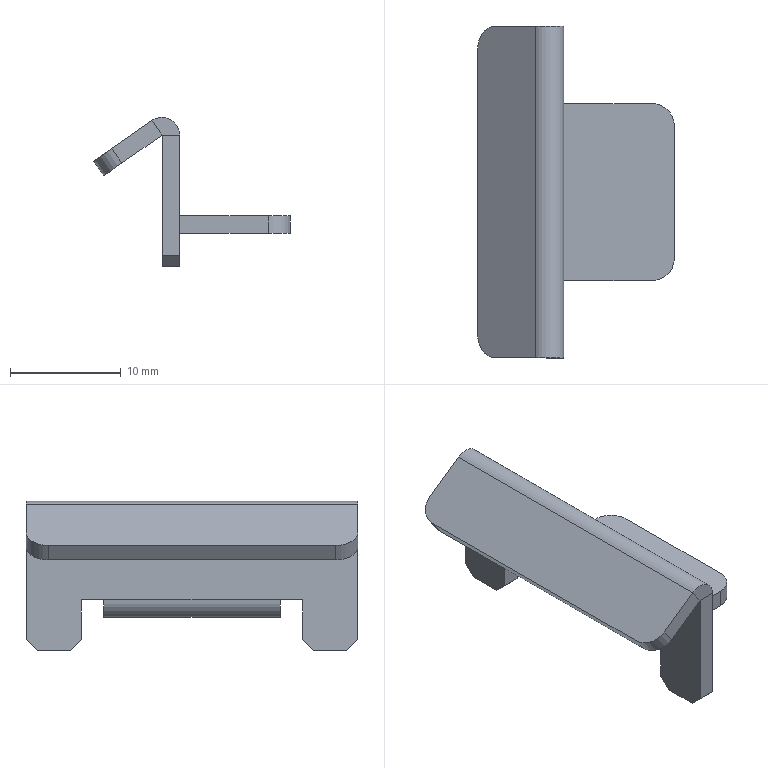Part | NX | features solid 2 | 1 solid | 34 faces | box 17.782 x 30 x 13.496 mm | volume 1096 mm3 | plane 28 | cylinder 6 | commonest cylinder face diameters 4 x4 3.2 x2
STEP:
#1=CARTESIAN_POINT('',(-290.6,942.6,-820.104));
#2=VERTEX_POINT('',#1);
#3=CARTESIAN_POINT('',(-290.6,942.6,-831.));
#4=VERTEX_POINT('',#3);
#5=CARTESIAN_POINT('',(-290.6,942.6,-820.104));
#6=DIRECTION('',(0.,0.,-1.));
#7=VECTOR('',#6,1000.);
#8=LINE('',#5,#7);
#9=EDGE_CURVE('',#2,#4,#8,.T.);
#10=ORIENTED_EDGE('',*,*,#9,.T.);
#11=CARTESIAN_POINT('',(-290.6,943.6,-832.));
#12=VERTEX_POINT('',#11);
#13=CARTESIAN_POINT('',(-290.6,943.6,-832.));
#14=DIRECTION('',(0.,-0.7071,0.7071));
#15=VECTOR('',#14,1000.);
#16=LINE('',#13,#15);
#17=EDGE_CURVE('',#12,#4,#16,.T.);
#18=ORIENTED_EDGE('',*,*,#17,.F.);
#19=CARTESIAN_POINT('',(-290.6,946.6,-832.));
#20=VERTEX_POINT('',#19);
#21=CARTESIAN_POINT('',(-290.6,943.6,-832.));
#22=DIRECTION('',(0.,1.,0.));
#23=VECTOR('',#22,1000.);
#24=LINE('',#21,#23);
#25=EDGE_CURVE('',#12,#20,#24,.T.);
#26=ORIENTED_EDGE('',*,*,#25,.T.);
#27=CARTESIAN_POINT('',(-290.6,947.6,-831.));
#28=VERTEX_POINT('',#27);
#29=CARTESIAN_POINT('',(-290.6,947.6,-831.));
#30=DIRECTION('',(0.,-0.7071,-0.7071));
#31=VECTOR('',#30,1000.);
#32=LINE('',#29,#31);
#33=EDGE_CURVE('',#28,#20,#32,.T.);
#34=ORIENTED_EDGE('',*,*,#33,.F.);
#35=CARTESIAN_POINT('',(-290.6,947.6,-827.4));
#36=VERTEX_POINT('',#35);
#37=CARTESIAN_POINT('',(-290.6,947.6,-831.));
#38=DIRECTION('',(0.,0.,1.));
#39=VECTOR('',#38,1000.);
#40=LINE('',#37,#39);
#41=EDGE_CURVE('',#28,#36,#40,.T.);
#42=ORIENTED_EDGE('',*,*,#41,.T.);
#43=CARTESIAN_POINT('',(-290.6,949.6,-827.4));
#44=VERTEX_POINT('',#43);
#45=CARTESIAN_POINT('',(-290.6,947.6,-827.4));
#46=DIRECTION('',(0.,1.,0.));
#47=VECTOR('',#46,1000.);
#48=LINE('',#45,#47);
#49=EDGE_CURVE('',#36,#44,#48,.T.);
#50=ORIENTED_EDGE('',*,*,#49,.T.);
#51=CARTESIAN_POINT('',(-290.6,965.6,-827.4));
#52=VERTEX_POINT('',#51);
#53=CARTESIAN_POINT('',(-290.6,949.6,-827.4));
#54=DIRECTION('',(0.,1.,0.));
#55=VECTOR('',#54,1000.);
#56=LINE('',#53,#55);
#57=EDGE_CURVE('',#44,#52,#56,.T.);
#58=ORIENTED_EDGE('',*,*,#57,.T.);
#59=CARTESIAN_POINT('',(-290.6,967.6,-827.4));
#60=VERTEX_POINT('',#59);
#61=CARTESIAN_POINT('',(-290.6,967.6,-827.4));
#62=DIRECTION('',(0.,-1.,0.));
#63=VECTOR('',#62,1000.);
#64=LINE('',#61,#63);
#65=EDGE_CURVE('',#60,#52,#64,.T.);
#66=ORIENTED_EDGE('',*,*,#65,.F.);
#67=CARTESIAN_POINT('',(-290.6,967.6,-831.));
#68=VERTEX_POINT('',#67);
#69=CARTESIAN_POINT('',(-290.6,967.6,-827.4));
#70=DIRECTION('',(0.,0.,-1.));
#71=VECTOR('',#70,1000.);
#72=LINE('',#69,#71);
#73=EDGE_CURVE('',#60,#68,#72,.T.);
#74=ORIENTED_EDGE('',*,*,#73,.T.);
#75=CARTESIAN_POINT('',(-290.6,968.6,-832.));
#76=VERTEX_POINT('',#75);
#77=CARTESIAN_POINT('',(-290.6,968.6,-832.));
#78=DIRECTION('',(0.,-0.7071,0.7071));
#79=VECTOR('',#78,1000.);
#80=LINE('',#77,#79);
#81=EDGE_CURVE('',#76,#68,#80,.T.);
#82=ORIENTED_EDGE('',*,*,#81,.F.);
#83=CARTESIAN_POINT('',(-290.6,971.6,-832.));
#84=VERTEX_POINT('',#83);
#85=CARTESIAN_POINT('',(-290.6,968.6,-832.));
#86=DIRECTION('',(0.,1.,0.));
#87=VECTOR('',#86,1000.);
#88=LINE('',#85,#87);
#89=EDGE_CURVE('',#76,#84,#88,.T.);
#90=ORIENTED_EDGE('',*,*,#89,.T.);
#91=CARTESIAN_POINT('',(-290.6,972.6,-831.));
#92=VERTEX_POINT('',#91);
#93=CARTESIAN_POINT('',(-290.6,972.6,-831.));
#94=DIRECTION('',(0.,-0.7071,-0.7071));
#95=VECTOR('',#94,1000.);
#96=LINE('',#93,#95);
#97=EDGE_CURVE('',#92,#84,#96,.T.);
#98=ORIENTED_EDGE('',*,*,#97,.F.);
#99=CARTESIAN_POINT('',(-290.6,972.6,-820.104));
#100=VERTEX_POINT('',#99);
#101=CARTESIAN_POINT('',(-290.6,972.6,-831.));
#102=DIRECTION('',(0.,0.,1.));
#103=VECTOR('',#102,1000.);
#104=LINE('',#101,#103);
#105=EDGE_CURVE('',#92,#100,#104,.T.);
#106=ORIENTED_EDGE('',*,*,#105,.T.);
#107=CARTESIAN_POINT('',(-290.6,972.6,-820.104));
#108=DIRECTION('',(0.,-1.,0.));
#109=VECTOR('',#108,1000.);
#110=LINE('',#107,#109);
#111=EDGE_CURVE('',#100,#2,#110,.T.);
#112=ORIENTED_EDGE('',*,*,#111,.T.);
#113=EDGE_LOOP('',(#10,#18,#26,#34,#42,#50,#58,#66,#74,#82,#90,#98,#106,#112));
#114=FACE_BOUND('',#113,.T.);
#115=CARTESIAN_POINT('',(-290.6,972.6,-817.03));
#116=DIRECTION('',(-1.,0.,0.));
#117=DIRECTION('',(0.,0.,1.));
#118=AXIS2_PLACEMENT_3D('',#115,#116,#117);
#119=PLANE('',#118);
#120=ADVANCED_FACE('',(#114),#119,.F.);
#121=ORIENTED_EDGE('',*,*,#111,.F.);
#122=CARTESIAN_POINT('',(-292.2,972.6,-818.504));
#123=VERTEX_POINT('',#122);
#124=CARTESIAN_POINT('',(-292.2,972.6,-820.104));
#125=DIRECTION('',(0.,-1.,0.));
#126=DIRECTION('',(1.,0.,0.));
#127=AXIS2_PLACEMENT_3D('',#124,#125,#126);
#128=CIRCLE('',#127,1.6);
#129=EDGE_CURVE('',#100,#123,#128,.T.);
#130=ORIENTED_EDGE('',*,*,#129,.T.);
#131=CARTESIAN_POINT('',(-293.118,972.6,-818.793));
#132=VERTEX_POINT('',#131);
#133=CARTESIAN_POINT('',(-292.2,972.6,-820.104));
#134=DIRECTION('',(0.,-1.,0.));
#135=DIRECTION('',(0.,0.,1.));
#136=AXIS2_PLACEMENT_3D('',#133,#134,#135);
#137=CIRCLE('',#136,1.6);
#138=EDGE_CURVE('',#123,#132,#137,.T.);
#139=ORIENTED_EDGE('',*,*,#138,.T.);
#140=CARTESIAN_POINT('',(-293.118,942.6,-818.793));
#141=VERTEX_POINT('',#140);
#142=CARTESIAN_POINT('',(-293.118,942.6,-818.793));
#143=DIRECTION('',(0.,1.,0.));
#144=VECTOR('',#143,1000.);
#145=LINE('',#142,#144);
#146=EDGE_CURVE('',#141,#132,#145,.T.);
#147=ORIENTED_EDGE('',*,*,#146,.F.);
#148=CARTESIAN_POINT('',(-292.2,942.6,-818.504));
#149=VERTEX_POINT('',#148);
#150=CARTESIAN_POINT('',(-292.2,942.6,-820.104));
#151=DIRECTION('',(0.,1.,0.));
#152=DIRECTION('',(-0.5736,0.,0.8192));
#153=AXIS2_PLACEMENT_3D('',#150,#151,#152);
#154=CIRCLE('',#153,1.6);
#155=EDGE_CURVE('',#141,#149,#154,.T.);
#156=ORIENTED_EDGE('',*,*,#155,.T.);
#157=CARTESIAN_POINT('',(-292.2,942.6,-820.104));
#158=DIRECTION('',(0.,1.,0.));
#159=DIRECTION('',(0.,0.,1.));
#160=AXIS2_PLACEMENT_3D('',#157,#158,#159);
#161=CIRCLE('',#160,1.6);
#162=EDGE_CURVE('',#149,#2,#161,.T.);
#163=ORIENTED_EDGE('',*,*,#162,.T.);
#164=EDGE_LOOP('',(#121,#130,#139,#147,#156,#163));
#165=FACE_BOUND('',#164,.T.);
#166=CARTESIAN_POINT('',(-292.2,942.6,-820.104));
#167=DIRECTION('',(0.,1.,0.));
#168=DIRECTION('',(0.,0.,-1.));
#169=AXIS2_PLACEMENT_3D('',#166,#167,#168);
#170=CYLINDRICAL_SURFACE('',#169,1.6);
#171=ADVANCED_FACE('',(#165),#170,.T.);
#172=CARTESIAN_POINT('',(-292.2,942.6,-820.104));
#173=VERTEX_POINT('',#172);
#174=CARTESIAN_POINT('',(-292.2,942.6,-820.104));
#175=DIRECTION('',(-0.5736,0.,0.8192));
#176=VECTOR('',#175,1000.);
#177=LINE('',#174,#176);
#178=EDGE_CURVE('',#173,#141,#177,.T.);
#179=ORIENTED_EDGE('',*,*,#178,.F.);
#180=CARTESIAN_POINT('',(-290.6,942.6,-820.104));
#181=DIRECTION('',(-1.,0.,0.));
#182=VECTOR('',#181,1000.);
#183=LINE('',#180,#182);
#184=EDGE_CURVE('',#2,#173,#183,.T.);
#185=ORIENTED_EDGE('',*,*,#184,.F.);
#186=ORIENTED_EDGE('',*,*,#162,.F.);
#187=ORIENTED_EDGE('',*,*,#155,.F.);
#188=EDGE_LOOP('',(#179,#185,#186,#187));
#189=FACE_BOUND('',#188,.T.);
#190=CARTESIAN_POINT('',(-291.831,942.6,-819.394));
#191=DIRECTION('',(0.,1.,0.));
#192=DIRECTION('',(0.,0.,-1.));
#193=AXIS2_PLACEMENT_3D('',#190,#191,#192);
#194=PLANE('',#193);
#195=ADVANCED_FACE('',(#189),#194,.F.);
#196=CARTESIAN_POINT('',(-292.2,942.6,-831.));
#197=VERTEX_POINT('',#196);
#198=CARTESIAN_POINT('',(-292.2,942.6,-831.));
#199=DIRECTION('',(0.,0.,1.));
#200=VECTOR('',#199,1000.);
#201=LINE('',#198,#200);
#202=EDGE_CURVE('',#197,#173,#201,.T.);
#203=ORIENTED_EDGE('',*,*,#202,.F.);
#204=CARTESIAN_POINT('',(-292.2,942.6,-831.));
#205=DIRECTION('',(1.,0.,0.));
#206=VECTOR('',#205,1000.);
#207=LINE('',#204,#206);
#208=EDGE_CURVE('',#197,#4,#207,.T.);
#209=ORIENTED_EDGE('',*,*,#208,.T.);
#210=ORIENTED_EDGE('',*,*,#9,.F.);
#211=ORIENTED_EDGE('',*,*,#184,.T.);
#212=EDGE_LOOP('',(#203,#209,#210,#211));
#213=FACE_BOUND('',#212,.T.);
#214=CARTESIAN_POINT('',(-291.4,942.6,-822.615));
#215=DIRECTION('',(0.,1.,0.));
#216=DIRECTION('',(0.,0.,1.));
#217=AXIS2_PLACEMENT_3D('',#214,#215,#216);
#218=PLANE('',#217);
#219=ADVANCED_FACE('',(#213),#218,.F.);
#220=ORIENTED_EDGE('',*,*,#208,.F.);
#221=CARTESIAN_POINT('',(-292.2,943.6,-832.));
#222=VERTEX_POINT('',#221);
#223=CARTESIAN_POINT('',(-292.2,942.6,-831.));
#224=DIRECTION('',(0.,0.7071,-0.7071));
#225=VECTOR('',#224,1000.);
#226=LINE('',#223,#225);
#227=EDGE_CURVE('',#197,#222,#226,.T.);
#228=ORIENTED_EDGE('',*,*,#227,.T.);
#229=CARTESIAN_POINT('',(-292.2,943.6,-832.));
#230=DIRECTION('',(1.,0.,0.));
#231=VECTOR('',#230,1000.);
#232=LINE('',#229,#231);
#233=EDGE_CURVE('',#222,#12,#232,.T.);
#234=ORIENTED_EDGE('',*,*,#233,.T.);
#235=ORIENTED_EDGE('',*,*,#17,.T.);
#236=EDGE_LOOP('',(#220,#228,#234,#235));
#237=FACE_BOUND('',#236,.T.);
#238=CARTESIAN_POINT('',(-291.4,943.1,-831.5));
#239=DIRECTION('',(0.,-0.7071,-0.7071));
#240=DIRECTION('',(0.,-0.7071,0.7071));
#241=AXIS2_PLACEMENT_3D('',#238,#239,#240);
#242=PLANE('',#241);
#243=ADVANCED_FACE('',(#237),#242,.T.);
#244=ORIENTED_EDGE('',*,*,#25,.F.);
#245=ORIENTED_EDGE('',*,*,#233,.F.);
#246=CARTESIAN_POINT('',(-292.2,946.6,-832.));
#247=VERTEX_POINT('',#246);
#248=CARTESIAN_POINT('',(-292.2,943.6,-832.));
#249=DIRECTION('',(0.,1.,0.));
#250=VECTOR('',#249,1000.);
#251=LINE('',#248,#250);
#252=EDGE_CURVE('',#222,#247,#251,.T.);
#253=ORIENTED_EDGE('',*,*,#252,.T.);
#254=CARTESIAN_POINT('',(-292.2,946.6,-832.));
#255=DIRECTION('',(1.,0.,0.));
#256=VECTOR('',#255,1000.);
#257=LINE('',#254,#256);
#258=EDGE_CURVE('',#247,#20,#257,.T.);
#259=ORIENTED_EDGE('',*,*,#258,.T.);
#260=EDGE_LOOP('',(#244,#245,#253,#259));
#261=FACE_BOUND('',#260,.T.);
#262=CARTESIAN_POINT('',(-291.4,945.1,-832.));
#263=DIRECTION('',(0.,0.,-1.));
#264=DIRECTION('',(0.,-1.,0.));
#265=AXIS2_PLACEMENT_3D('',#262,#263,#264);
#266=PLANE('',#265);
#267=ADVANCED_FACE('',(#261),#266,.T.);
#268=ORIENTED_EDGE('',*,*,#258,.F.);
#269=CARTESIAN_POINT('',(-292.2,947.6,-831.));
#270=VERTEX_POINT('',#269);
#271=CARTESIAN_POINT('',(-292.2,946.6,-832.));
#272=DIRECTION('',(0.,0.7071,0.7071));
#273=VECTOR('',#272,1000.);
#274=LINE('',#271,#273);
#275=EDGE_CURVE('',#247,#270,#274,.T.);
#276=ORIENTED_EDGE('',*,*,#275,.T.);
#277=CARTESIAN_POINT('',(-292.2,947.6,-831.));
#278=DIRECTION('',(1.,0.,0.));
#279=VECTOR('',#278,1000.);
#280=LINE('',#277,#279);
#281=EDGE_CURVE('',#270,#28,#280,.T.);
#282=ORIENTED_EDGE('',*,*,#281,.T.);
#283=ORIENTED_EDGE('',*,*,#33,.T.);
#284=EDGE_LOOP('',(#268,#276,#282,#283));
#285=FACE_BOUND('',#284,.T.);
#286=CARTESIAN_POINT('',(-291.4,947.1,-831.5));
#287=DIRECTION('',(0.,0.7071,-0.7071));
#288=DIRECTION('',(0.,-0.7071,-0.7071));
#289=AXIS2_PLACEMENT_3D('',#286,#287,#288);
#290=PLANE('',#289);
#291=ADVANCED_FACE('',(#285),#290,.T.);
#292=CARTESIAN_POINT('',(-292.2,947.6,-827.4));
#293=VERTEX_POINT('',#292);
#294=CARTESIAN_POINT('',(-292.2,947.6,-831.));
#295=DIRECTION('',(0.,0.,1.));
#296=VECTOR('',#295,1000.);
#297=LINE('',#294,#296);
#298=EDGE_CURVE('',#270,#293,#297,.T.);
#299=ORIENTED_EDGE('',*,*,#298,.T.);
#300=CARTESIAN_POINT('',(-290.6,947.6,-827.4));
#301=DIRECTION('',(-1.,0.,0.));
#302=VECTOR('',#301,1000.);
#303=LINE('',#300,#302);
#304=EDGE_CURVE('',#36,#293,#303,.T.);
#305=ORIENTED_EDGE('',*,*,#304,.F.);
#306=ORIENTED_EDGE('',*,*,#41,.F.);
#307=ORIENTED_EDGE('',*,*,#281,.F.);
#308=EDGE_LOOP('',(#299,#305,#306,#307));
#309=FACE_BOUND('',#308,.T.);
#310=CARTESIAN_POINT('',(-291.4,947.6,-829.7));
#311=DIRECTION('',(0.,1.,0.));
#312=DIRECTION('',(0.,0.,-1.));
#313=AXIS2_PLACEMENT_3D('',#310,#311,#312);
#314=PLANE('',#313);
#315=ADVANCED_FACE('',(#309),#314,.T.);
#316=CARTESIAN_POINT('',(-292.2,949.6,-827.4));
#317=VERTEX_POINT('',#316);
#318=CARTESIAN_POINT('',(-292.2,947.6,-827.4));
#319=DIRECTION('',(0.,1.,0.));
#320=VECTOR('',#319,1000.);
#321=LINE('',#318,#320);
#322=EDGE_CURVE('',#293,#317,#321,.T.);
#323=ORIENTED_EDGE('',*,*,#322,.T.);
#324=CARTESIAN_POINT('',(-292.2,949.6,-827.4));
#325=DIRECTION('',(1.,0.,0.));
#326=VECTOR('',#325,1000.);
#327=LINE('',#324,#326);
#328=EDGE_CURVE('',#317,#44,#327,.T.);
#329=ORIENTED_EDGE('',*,*,#328,.T.);
#330=ORIENTED_EDGE('',*,*,#49,.F.);
#331=ORIENTED_EDGE('',*,*,#304,.T.);
#332=EDGE_LOOP('',(#323,#329,#330,#331));
#333=FACE_BOUND('',#332,.T.);
#334=CARTESIAN_POINT('',(-291.4,946.1,-827.4));
#335=DIRECTION('',(0.,0.,1.));
#336=DIRECTION('',(0.,-1.,0.));
#337=AXIS2_PLACEMENT_3D('',#334,#335,#336);
#338=PLANE('',#337);
#339=ADVANCED_FACE('',(#333),#338,.F.);
#340=ORIENTED_EDGE('',*,*,#328,.F.);
#341=CARTESIAN_POINT('',(-290.6,949.6,-829.));
#342=VERTEX_POINT('',#341);
#343=CARTESIAN_POINT('',(-290.6,949.6,-827.4));
#344=DIRECTION('',(0.,1.,0.));
#345=DIRECTION('',(0.,0.,-1.));
#346=AXIS2_PLACEMENT_3D('',#343,#344,#345);
#347=CIRCLE('',#346,1.6);
#348=EDGE_CURVE('',#342,#317,#347,.T.);
#349=ORIENTED_EDGE('',*,*,#348,.F.);
#350=CARTESIAN_POINT('',(-290.6,949.6,-829.));
#351=DIRECTION('',(0.,0.,1.));
#352=VECTOR('',#351,1000.);
#353=LINE('',#350,#352);
#354=EDGE_CURVE('',#342,#44,#353,.T.);
#355=ORIENTED_EDGE('',*,*,#354,.T.);
#356=EDGE_LOOP('',(#340,#349,#355));
#357=FACE_BOUND('',#356,.T.);
#358=CARTESIAN_POINT('',(-291.166,949.6,-827.966));
#359=DIRECTION('',(0.,-1.,0.));
#360=DIRECTION('',(1.,0.,0.));
#361=AXIS2_PLACEMENT_3D('',#358,#359,#360);
#362=PLANE('',#361);
#363=ADVANCED_FACE('',(#357),#362,.T.);
#364=CARTESIAN_POINT('',(-282.6,949.6,-827.4));
#365=VERTEX_POINT('',#364);
#366=CARTESIAN_POINT('',(-290.6,949.6,-827.4));
#367=DIRECTION('',(1.,0.,0.));
#368=VECTOR('',#367,1000.);
#369=LINE('',#366,#368);
#370=EDGE_CURVE('',#44,#365,#369,.T.);
#371=ORIENTED_EDGE('',*,*,#370,.F.);
#372=ORIENTED_EDGE('',*,*,#354,.F.);
#373=CARTESIAN_POINT('',(-282.6,949.6,-829.));
#374=VERTEX_POINT('',#373);
#375=CARTESIAN_POINT('',(-290.6,949.6,-829.));
#376=DIRECTION('',(1.,0.,0.));
#377=VECTOR('',#376,1000.);
#378=LINE('',#375,#377);
#379=EDGE_CURVE('',#342,#374,#378,.T.);
#380=ORIENTED_EDGE('',*,*,#379,.T.);
#381=CARTESIAN_POINT('',(-282.6,949.6,-829.));
#382=DIRECTION('',(0.,0.,1.));
#383=VECTOR('',#382,1000.);
#384=LINE('',#381,#383);
#385=EDGE_CURVE('',#374,#365,#384,.T.);
#386=ORIENTED_EDGE('',*,*,#385,.T.);
#387=EDGE_LOOP('',(#371,#372,#380,#386));
#388=FACE_BOUND('',#387,.T.);
#389=CARTESIAN_POINT('',(-285.6,949.6,-828.2));
#390=DIRECTION('',(0.,1.,0.));
#391=DIRECTION('',(-1.,0.,0.));
#392=AXIS2_PLACEMENT_3D('',#389,#390,#391);
#393=PLANE('',#392);
#394=ADVANCED_FACE('',(#388),#393,.F.);
#395=CARTESIAN_POINT('',(-280.6,951.6,-827.4));
#396=VERTEX_POINT('',#395);
#397=CARTESIAN_POINT('',(-280.6,951.6,-829.));
#398=VERTEX_POINT('',#397);
#399=CARTESIAN_POINT('',(-280.6,951.6,-827.4));
#400=DIRECTION('',(0.,0.,-1.));
#401=VECTOR('',#400,1000.);
#402=LINE('',#399,#401);
#403=EDGE_CURVE('',#396,#398,#402,.T.);
#404=ORIENTED_EDGE('',*,*,#403,.F.);
#405=CARTESIAN_POINT('',(-282.6,951.6,-827.4));
#406=DIRECTION('',(0.,0.,-1.));
#407=DIRECTION('',(1.,0.,0.));
#408=AXIS2_PLACEMENT_3D('',#405,#406,#407);
#409=CIRCLE('',#408,2.);
#410=EDGE_CURVE('',#396,#365,#409,.T.);
#411=ORIENTED_EDGE('',*,*,#410,.T.);
#412=ORIENTED_EDGE('',*,*,#385,.F.);
#413=CARTESIAN_POINT('',(-282.6,951.6,-829.));
#414=DIRECTION('',(0.,0.,1.));
#415=DIRECTION('',(0.,-1.,0.));
#416=AXIS2_PLACEMENT_3D('',#413,#414,#415);
#417=CIRCLE('',#416,2.);
#418=EDGE_CURVE('',#374,#398,#417,.T.);
#419=ORIENTED_EDGE('',*,*,#418,.T.);
#420=EDGE_LOOP('',(#404,#411,#412,#419));
#421=FACE_BOUND('',#420,.T.);
#422=CARTESIAN_POINT('',(-282.6,951.6,-800.897));
#423=DIRECTION('',(0.,0.,-1.));
#424=DIRECTION('',(-1.,0.,0.));
#425=AXIS2_PLACEMENT_3D('',#422,#423,#424);
#426=CYLINDRICAL_SURFACE('',#425,2.);
#427=ADVANCED_FACE('',(#421),#426,.T.);
#428=CARTESIAN_POINT('',(-280.6,963.6,-829.));
#429=VERTEX_POINT('',#428);
#430=CARTESIAN_POINT('',(-280.6,963.6,-829.));
#431=DIRECTION('',(0.,-1.,0.));
#432=VECTOR('',#431,1000.);
#433=LINE('',#430,#432);
#434=EDGE_CURVE('',#429,#398,#433,.T.);
#435=ORIENTED_EDGE('',*,*,#434,.T.);
#436=ORIENTED_EDGE('',*,*,#418,.F.);
#437=ORIENTED_EDGE('',*,*,#379,.F.);
#438=CARTESIAN_POINT('',(-290.6,965.6,-829.));
#439=VERTEX_POINT('',#438);
#440=CARTESIAN_POINT('',(-290.6,949.6,-829.));
#441=DIRECTION('',(0.,1.,0.));
#442=VECTOR('',#441,1000.);
#443=LINE('',#440,#442);
#444=EDGE_CURVE('',#342,#439,#443,.T.);
#445=ORIENTED_EDGE('',*,*,#444,.T.);
#446=CARTESIAN_POINT('',(-282.6,965.6,-829.));
#447=VERTEX_POINT('',#446);
#448=CARTESIAN_POINT('',(-290.6,965.6,-829.));
#449=DIRECTION('',(1.,0.,0.));
#450=VECTOR('',#449,1000.);
#451=LINE('',#448,#450);
#452=EDGE_CURVE('',#439,#447,#451,.T.);
#453=ORIENTED_EDGE('',*,*,#452,.T.);
#454=CARTESIAN_POINT('',(-282.6,963.6,-829.));
#455=DIRECTION('',(0.,0.,1.));
#456=DIRECTION('',(1.,0.,0.));
#457=AXIS2_PLACEMENT_3D('',#454,#455,#456);
#458=CIRCLE('',#457,2.);
#459=EDGE_CURVE('',#429,#447,#458,.T.);
#460=ORIENTED_EDGE('',*,*,#459,.F.);
#461=EDGE_LOOP('',(#435,#436,#437,#445,#453,#460));
#462=FACE_BOUND('',#461,.T.);
#463=CARTESIAN_POINT('',(-292.2,972.6,-829.));
#464=DIRECTION('',(0.,0.,-1.));
#465=DIRECTION('',(-1.,0.,0.));
#466=AXIS2_PLACEMENT_3D('',#463,#464,#465);
#467=PLANE('',#466);
#468=ADVANCED_FACE('',(#462),#467,.T.);
#469=CARTESIAN_POINT('',(-282.6,965.6,-827.4));
#470=VERTEX_POINT('',#469);
#471=CARTESIAN_POINT('',(-282.6,965.6,-827.4));
#472=DIRECTION('',(0.,0.,-1.));
#473=VECTOR('',#472,1000.);
#474=LINE('',#471,#473);
#475=EDGE_CURVE('',#470,#447,#474,.T.);
#476=ORIENTED_EDGE('',*,*,#475,.F.);
#477=CARTESIAN_POINT('',(-280.6,963.6,-827.4));
#478=VERTEX_POINT('',#477);
#479=CARTESIAN_POINT('',(-282.6,963.6,-827.4));
#480=DIRECTION('',(0.,0.,-1.));
#481=DIRECTION('',(0.,1.,0.));
#482=AXIS2_PLACEMENT_3D('',#479,#480,#481);
#483=CIRCLE('',#482,2.);
#484=EDGE_CURVE('',#470,#478,#483,.T.);
#485=ORIENTED_EDGE('',*,*,#484,.T.);
#486=CARTESIAN_POINT('',(-280.6,963.6,-829.));
#487=DIRECTION('',(0.,0.,1.));
#488=VECTOR('',#487,1000.);
#489=LINE('',#486,#488);
#490=EDGE_CURVE('',#429,#478,#489,.T.);
#491=ORIENTED_EDGE('',*,*,#490,.F.);
#492=ORIENTED_EDGE('',*,*,#459,.T.);
#493=EDGE_LOOP('',(#476,#485,#491,#492));
#494=FACE_BOUND('',#493,.T.);
#495=CARTESIAN_POINT('',(-282.6,963.6,-800.897));
#496=DIRECTION('',(0.,0.,-1.));
#497=DIRECTION('',(0.,-1.,0.));
#498=AXIS2_PLACEMENT_3D('',#495,#496,#497);
#499=CYLINDRICAL_SURFACE('',#498,2.);
#500=ADVANCED_FACE('',(#494),#499,.T.);
#501=CARTESIAN_POINT('',(-280.6,963.6,-827.4));
#502=DIRECTION('',(0.,-1.,0.));
#503=VECTOR('',#502,1000.);
#504=LINE('',#501,#503);
#505=EDGE_CURVE('',#478,#396,#504,.T.);
#506=ORIENTED_EDGE('',*,*,#505,.T.);
#507=ORIENTED_EDGE('',*,*,#403,.T.);
#508=ORIENTED_EDGE('',*,*,#434,.F.);
#509=ORIENTED_EDGE('',*,*,#490,.T.);
#510=EDGE_LOOP('',(#506,#507,#508,#509));
#511=FACE_BOUND('',#510,.T.);
#512=CARTESIAN_POINT('',(-280.6,957.6,-828.2));
#513=DIRECTION('',(1.,0.,0.));
#514=DIRECTION('',(0.,1.,0.));
#515=AXIS2_PLACEMENT_3D('',#512,#513,#514);
#516=PLANE('',#515);
#517=ADVANCED_FACE('',(#511),#516,.T.);
#518=CARTESIAN_POINT('',(-290.6,965.6,-827.4));
#519=DIRECTION('',(1.,0.,0.));
#520=VECTOR('',#519,1000.);
#521=LINE('',#518,#520);
#522=EDGE_CURVE('',#52,#470,#521,.T.);
#523=ORIENTED_EDGE('',*,*,#522,.F.);
#524=ORIENTED_EDGE('',*,*,#57,.F.);
#525=ORIENTED_EDGE('',*,*,#370,.T.);
#526=ORIENTED_EDGE('',*,*,#410,.F.);
#527=ORIENTED_EDGE('',*,*,#505,.F.);
#528=ORIENTED_EDGE('',*,*,#484,.F.);
#529=EDGE_LOOP('',(#523,#524,#525,#526,#527,#528));
#530=FACE_BOUND('',#529,.T.);
#531=CARTESIAN_POINT('',(-292.2,972.6,-827.4));
#532=DIRECTION('',(0.,0.,-1.));
#533=DIRECTION('',(-1.,0.,0.));
#534=AXIS2_PLACEMENT_3D('',#531,#532,#533);
#535=PLANE('',#534);
#536=ADVANCED_FACE('',(#530),#535,.F.);
#537=ORIENTED_EDGE('',*,*,#452,.F.);
#538=CARTESIAN_POINT('',(-290.6,965.6,-829.));
#539=DIRECTION('',(0.,0.,1.));
#540=VECTOR('',#539,1000.);
#541=LINE('',#538,#540);
#542=EDGE_CURVE('',#439,#52,#541,.T.);
#543=ORIENTED_EDGE('',*,*,#542,.T.);
#544=ORIENTED_EDGE('',*,*,#522,.T.);
#545=ORIENTED_EDGE('',*,*,#475,.T.);
#546=EDGE_LOOP('',(#537,#543,#544,#545));
#547=FACE_BOUND('',#546,.T.);
#548=CARTESIAN_POINT('',(-285.6,965.6,-828.2));
#549=DIRECTION('',(0.,1.,0.));
#550=DIRECTION('',(-1.,0.,0.));
#551=AXIS2_PLACEMENT_3D('',#548,#549,#550);
#552=PLANE('',#551);
#553=ADVANCED_FACE('',(#547),#552,.T.);
#554=ORIENTED_EDGE('',*,*,#542,.F.);
#555=CARTESIAN_POINT('',(-292.2,965.6,-827.4));
#556=VERTEX_POINT('',#555);
#557=CARTESIAN_POINT('',(-290.6,965.6,-827.4));
#558=DIRECTION('',(0.,-1.,0.));
#559=DIRECTION('',(-1.,0.,0.));
#560=AXIS2_PLACEMENT_3D('',#557,#558,#559);
#561=CIRCLE('',#560,1.6);
#562=EDGE_CURVE('',#556,#439,#561,.T.);
#563=ORIENTED_EDGE('',*,*,#562,.F.);
#564=CARTESIAN_POINT('',(-292.2,965.6,-827.4));
#565=DIRECTION('',(1.,0.,0.));
#566=VECTOR('',#565,1000.);
#567=LINE('',#564,#566);
#568=EDGE_CURVE('',#556,#52,#567,.T.);
#569=ORIENTED_EDGE('',*,*,#568,.T.);
#570=EDGE_LOOP('',(#554,#563,#569));
#571=FACE_BOUND('',#570,.T.);
#572=CARTESIAN_POINT('',(-291.166,965.6,-827.966));
#573=DIRECTION('',(0.,-1.,0.));
#574=DIRECTION('',(1.,0.,0.));
#575=AXIS2_PLACEMENT_3D('',#572,#573,#574);
#576=PLANE('',#575);
#577=ADVANCED_FACE('',(#571),#576,.F.);
#578=ORIENTED_EDGE('',*,*,#65,.T.);
#579=ORIENTED_EDGE('',*,*,#568,.F.);
#580=CARTESIAN_POINT('',(-292.2,967.6,-827.4));
#581=VERTEX_POINT('',#580);
#582=CARTESIAN_POINT('',(-292.2,967.6,-827.4));
#583=DIRECTION('',(0.,-1.,0.));
#584=VECTOR('',#583,1000.);
#585=LINE('',#582,#584);
#586=EDGE_CURVE('',#581,#556,#585,.T.);
#587=ORIENTED_EDGE('',*,*,#586,.F.);
#588=CARTESIAN_POINT('',(-290.6,967.6,-827.4));
#589=DIRECTION('',(-1.,0.,0.));
#590=VECTOR('',#589,1000.);
#591=LINE('',#588,#590);
#592=EDGE_CURVE('',#60,#581,#591,.T.);
#593=ORIENTED_EDGE('',*,*,#592,.F.);
#594=EDGE_LOOP('',(#578,#579,#587,#593));
#595=FACE_BOUND('',#594,.T.);
#596=CARTESIAN_POINT('',(-291.4,969.1,-827.4));
#597=DIRECTION('',(0.,0.,-1.));
#598=DIRECTION('',(0.,1.,0.));
#599=AXIS2_PLACEMENT_3D('',#596,#597,#598);
#600=PLANE('',#599);
#601=ADVANCED_FACE('',(#595),#600,.T.);
#602=ORIENTED_EDGE('',*,*,#73,.F.);
#603=ORIENTED_EDGE('',*,*,#592,.T.);
#604=CARTESIAN_POINT('',(-292.2,967.6,-831.));
#605=VERTEX_POINT('',#604);
#606=CARTESIAN_POINT('',(-292.2,967.6,-827.4));
#607=DIRECTION('',(0.,0.,-1.));
#608=VECTOR('',#607,1000.);
#609=LINE('',#606,#608);
#610=EDGE_CURVE('',#581,#605,#609,.T.);
#611=ORIENTED_EDGE('',*,*,#610,.T.);
#612=CARTESIAN_POINT('',(-292.2,967.6,-831.));
#613=DIRECTION('',(1.,0.,0.));
#614=VECTOR('',#613,1000.);
#615=LINE('',#612,#614);
#616=EDGE_CURVE('',#605,#68,#615,.T.);
#617=ORIENTED_EDGE('',*,*,#616,.T.);
#618=EDGE_LOOP('',(#602,#603,#611,#617));
#619=FACE_BOUND('',#618,.T.);
#620=CARTESIAN_POINT('',(-291.4,967.6,-829.7));
#621=DIRECTION('',(0.,-1.,0.));
#622=DIRECTION('',(0.,0.,1.));
#623=AXIS2_PLACEMENT_3D('',#620,#621,#622);
#624=PLANE('',#623);
#625=ADVANCED_FACE('',(#619),#624,.T.);
#626=ORIENTED_EDGE('',*,*,#616,.F.);
#627=CARTESIAN_POINT('',(-292.2,968.6,-832.));
#628=VERTEX_POINT('',#627);
#629=CARTESIAN_POINT('',(-292.2,967.6,-831.));
#630=DIRECTION('',(0.,0.7071,-0.7071));
#631=VECTOR('',#630,1000.);
#632=LINE('',#629,#631);
#633=EDGE_CURVE('',#605,#628,#632,.T.);
#634=ORIENTED_EDGE('',*,*,#633,.T.);
#635=CARTESIAN_POINT('',(-292.2,968.6,-832.));
#636=DIRECTION('',(1.,0.,0.));
#637=VECTOR('',#636,1000.);
#638=LINE('',#635,#637);
#639=EDGE_CURVE('',#628,#76,#638,.T.);
#640=ORIENTED_EDGE('',*,*,#639,.T.);
#641=ORIENTED_EDGE('',*,*,#81,.T.);
#642=EDGE_LOOP('',(#626,#634,#640,#641));
#643=FACE_BOUND('',#642,.T.);
#644=CARTESIAN_POINT('',(-291.4,968.1,-831.5));
#645=DIRECTION('',(0.,-0.7071,-0.7071));
#646=DIRECTION('',(0.,-0.7071,0.7071));
#647=AXIS2_PLACEMENT_3D('',#644,#645,#646);
#648=PLANE('',#647);
#649=ADVANCED_FACE('',(#643),#648,.T.);
#650=CARTESIAN_POINT('',(-292.2,971.6,-832.));
#651=VERTEX_POINT('',#650);
#652=CARTESIAN_POINT('',(-292.2,968.6,-832.));
#653=DIRECTION('',(0.,1.,0.));
#654=VECTOR('',#653,1000.);
#655=LINE('',#652,#654);
#656=EDGE_CURVE('',#628,#651,#655,.T.);
#657=ORIENTED_EDGE('',*,*,#656,.T.);
#658=CARTESIAN_POINT('',(-292.2,971.6,-832.));
#659=DIRECTION('',(1.,0.,0.));
#660=VECTOR('',#659,1000.);
#661=LINE('',#658,#660);
#662=EDGE_CURVE('',#651,#84,#661,.T.);
#663=ORIENTED_EDGE('',*,*,#662,.T.);
#664=ORIENTED_EDGE('',*,*,#89,.F.);
#665=ORIENTED_EDGE('',*,*,#639,.F.);
#666=EDGE_LOOP('',(#657,#663,#664,#665));
#667=FACE_BOUND('',#666,.T.);
#668=CARTESIAN_POINT('',(-291.4,970.1,-832.));
#669=DIRECTION('',(0.,0.,-1.));
#670=DIRECTION('',(0.,-1.,0.));
#671=AXIS2_PLACEMENT_3D('',#668,#669,#670);
#672=PLANE('',#671);
#673=ADVANCED_FACE('',(#667),#672,.T.);
#674=ORIENTED_EDGE('',*,*,#662,.F.);
#675=CARTESIAN_POINT('',(-292.2,972.6,-831.));
#676=VERTEX_POINT('',#675);
#677=CARTESIAN_POINT('',(-292.2,971.6,-832.));
#678=DIRECTION('',(0.,0.7071,0.7071));
#679=VECTOR('',#678,1000.);
#680=LINE('',#677,#679);
#681=EDGE_CURVE('',#651,#676,#680,.T.);
#682=ORIENTED_EDGE('',*,*,#681,.T.);
#683=CARTESIAN_POINT('',(-292.2,972.6,-831.));
#684=DIRECTION('',(1.,0.,0.));
#685=VECTOR('',#684,1000.);
#686=LINE('',#683,#685);
#687=EDGE_CURVE('',#676,#92,#686,.T.);
#688=ORIENTED_EDGE('',*,*,#687,.T.);
#689=ORIENTED_EDGE('',*,*,#97,.T.);
#690=EDGE_LOOP('',(#674,#682,#688,#689));
#691=FACE_BOUND('',#690,.T.);
#692=CARTESIAN_POINT('',(-291.4,972.1,-831.5));
#693=DIRECTION('',(0.,0.7071,-0.7071));
#694=DIRECTION('',(0.,-0.7071,-0.7071));
#695=AXIS2_PLACEMENT_3D('',#692,#693,#694);
#696=PLANE('',#695);
#697=ADVANCED_FACE('',(#691),#696,.T.);
#698=ORIENTED_EDGE('',*,*,#105,.F.);
#699=ORIENTED_EDGE('',*,*,#687,.F.);
#700=CARTESIAN_POINT('',(-292.2,972.6,-820.104));
#701=VERTEX_POINT('',#700);
#702=CARTESIAN_POINT('',(-292.2,972.6,-820.104));
#703=DIRECTION('',(0.,0.,-1.));
#704=VECTOR('',#703,1000.);
#705=LINE('',#702,#704);
#706=EDGE_CURVE('',#701,#676,#705,.T.);
#707=ORIENTED_EDGE('',*,*,#706,.F.);
#708=CARTESIAN_POINT('',(-290.6,972.6,-820.104));
#709=DIRECTION('',(-1.,0.,0.));
#710=VECTOR('',#709,1000.);
#711=LINE('',#708,#710);
#712=EDGE_CURVE('',#100,#701,#711,.T.);
#713=ORIENTED_EDGE('',*,*,#712,.F.);
#714=EDGE_LOOP('',(#698,#699,#707,#713));
#715=FACE_BOUND('',#714,.T.);
#716=CARTESIAN_POINT('',(-291.4,972.6,-822.615));
#717=DIRECTION('',(0.,1.,0.));
#718=DIRECTION('',(0.,0.,1.));
#719=AXIS2_PLACEMENT_3D('',#716,#717,#718);
#720=PLANE('',#719);
#721=ADVANCED_FACE('',(#715),#720,.T.);
#722=ORIENTED_EDGE('',*,*,#712,.T.);
#723=CARTESIAN_POINT('',(-293.118,972.6,-818.793));
#724=DIRECTION('',(0.5736,0.,-0.8192));
#725=VECTOR('',#724,1000.);
#726=LINE('',#723,#725);
#727=EDGE_CURVE('',#132,#701,#726,.T.);
#728=ORIENTED_EDGE('',*,*,#727,.F.);
#729=ORIENTED_EDGE('',*,*,#138,.F.);
#730=ORIENTED_EDGE('',*,*,#129,.F.);
#731=EDGE_LOOP('',(#722,#728,#729,#730));
#732=FACE_BOUND('',#731,.T.);
#733=CARTESIAN_POINT('',(-291.831,972.6,-819.394));
#734=DIRECTION('',(0.,1.,0.));
#735=DIRECTION('',(0.,0.,-1.));
#736=AXIS2_PLACEMENT_3D('',#733,#734,#735);
#737=PLANE('',#736);
#738=ADVANCED_FACE('',(#732),#737,.T.);
#739=CARTESIAN_POINT('',(-296.744,972.6,-821.332));
#740=VERTEX_POINT('',#739);
#741=CARTESIAN_POINT('',(-293.118,972.6,-818.793));
#742=DIRECTION('',(-0.8192,0.,-0.5736));
#743=VECTOR('',#742,1000.);
#744=LINE('',#741,#743);
#745=EDGE_CURVE('',#132,#740,#744,.T.);
#746=ORIENTED_EDGE('',*,*,#745,.F.);
#747=ORIENTED_EDGE('',*,*,#727,.T.);
#748=CARTESIAN_POINT('',(-295.826,972.6,-822.642));
#749=VERTEX_POINT('',#748);
#750=CARTESIAN_POINT('',(-292.2,972.6,-820.104));
#751=DIRECTION('',(-0.8192,0.,-0.5736));
#752=VECTOR('',#751,1000.);
#753=LINE('',#750,#752);
#754=EDGE_CURVE('',#701,#749,#753,.T.);
#755=ORIENTED_EDGE('',*,*,#754,.T.);
#756=CARTESIAN_POINT('',(-295.826,972.6,-822.642));
#757=DIRECTION('',(-0.5736,0.,0.8192));
#758=VECTOR('',#757,1000.);
#759=LINE('',#756,#758);
#760=EDGE_CURVE('',#749,#740,#759,.T.);
#761=ORIENTED_EDGE('',*,*,#760,.T.);
#762=EDGE_LOOP('',(#746,#747,#755,#761));
#763=FACE_BOUND('',#762,.T.);
#764=CARTESIAN_POINT('',(-295.291,972.6,-821.291));
#765=DIRECTION('',(0.,1.,0.));
#766=DIRECTION('',(0.8192,0.,0.5736));
#767=AXIS2_PLACEMENT_3D('',#764,#765,#766);
#768=PLANE('',#767);
#769=ADVANCED_FACE('',(#763),#768,.T.);
#770=ORIENTED_EDGE('',*,*,#760,.F.);
#771=CARTESIAN_POINT('',(-297.464,970.6,-823.79));
#772=VERTEX_POINT('',#771);
#773=CARTESIAN_POINT('',(-295.826,970.6,-822.642));
#774=DIRECTION('',(-0.5736,0.,0.8192));
#775=DIRECTION('',(0.,1.,0.));
#776=AXIS2_PLACEMENT_3D('',#773,#774,#775);
#777=CIRCLE('',#776,2.);
#778=EDGE_CURVE('',#749,#772,#777,.T.);
#779=ORIENTED_EDGE('',*,*,#778,.T.);
#780=CARTESIAN_POINT('',(-298.382,970.6,-822.479));
#781=VERTEX_POINT('',#780);
#782=CARTESIAN_POINT('',(-298.382,970.6,-822.479));
#783=DIRECTION('',(0.5736,0.,-0.8192));
#784=VECTOR('',#783,1000.);
#785=LINE('',#782,#784);
#786=EDGE_CURVE('',#781,#772,#785,.T.);
#787=ORIENTED_EDGE('',*,*,#786,.F.);
#788=CARTESIAN_POINT('',(-296.744,970.6,-821.332));
#789=DIRECTION('',(0.5736,0.,-0.8192));
#790=DIRECTION('',(-0.8192,0.,-0.5736));
#791=AXIS2_PLACEMENT_3D('',#788,#789,#790);
#792=CIRCLE('',#791,2.);
#793=EDGE_CURVE('',#781,#740,#792,.T.);
#794=ORIENTED_EDGE('',*,*,#793,.T.);
#795=EDGE_LOOP('',(#770,#779,#787,#794));
#796=FACE_BOUND('',#795,.T.);
#797=CARTESIAN_POINT('',(-276.949,970.6,-849.601));
#798=DIRECTION('',(-0.5736,0.,0.8192));
#799=DIRECTION('',(0.,-1.,0.));
#800=AXIS2_PLACEMENT_3D('',#797,#798,#799);
#801=CYLINDRICAL_SURFACE('',#800,2.);
#802=ADVANCED_FACE('',(#796),#801,.T.);
#803=CARTESIAN_POINT('',(-298.382,944.6,-822.479));
#804=VERTEX_POINT('',#803);
#805=CARTESIAN_POINT('',(-298.382,944.6,-822.479));
#806=DIRECTION('',(0.,1.,0.));
#807=VECTOR('',#806,1000.);
#808=LINE('',#805,#807);
#809=EDGE_CURVE('',#804,#781,#808,.T.);
#810=ORIENTED_EDGE('',*,*,#809,.F.);
#811=CARTESIAN_POINT('',(-296.744,942.6,-821.332));
#812=VERTEX_POINT('',#811);
#813=CARTESIAN_POINT('',(-296.744,944.6,-821.332));
#814=DIRECTION('',(0.5736,0.,-0.8192));
#815=DIRECTION('',(0.,-1.,0.));
#816=AXIS2_PLACEMENT_3D('',#813,#814,#815);
#817=CIRCLE('',#816,2.);
#818=EDGE_CURVE('',#812,#804,#817,.T.);
#819=ORIENTED_EDGE('',*,*,#818,.F.);
#820=CARTESIAN_POINT('',(-293.118,942.6,-818.793));
#821=DIRECTION('',(-0.8192,0.,-0.5736));
#822=VECTOR('',#821,1000.);
#823=LINE('',#820,#822);
#824=EDGE_CURVE('',#141,#812,#823,.T.);
#825=ORIENTED_EDGE('',*,*,#824,.F.);
#826=ORIENTED_EDGE('',*,*,#146,.T.);
#827=ORIENTED_EDGE('',*,*,#745,.T.);
#828=ORIENTED_EDGE('',*,*,#793,.F.);
#829=EDGE_LOOP('',(#810,#819,#825,#826,#827,#828));
#830=FACE_BOUND('',#829,.T.);
#831=CARTESIAN_POINT('',(-293.118,942.6,-818.793));
#832=DIRECTION('',(0.5736,0.,-0.8192));
#833=DIRECTION('',(0.8192,0.,0.5736));
#834=AXIS2_PLACEMENT_3D('',#831,#832,#833);
#835=PLANE('',#834);
#836=ADVANCED_FACE('',(#830),#835,.F.);
#837=CARTESIAN_POINT('',(-295.826,942.6,-822.642));
#838=VERTEX_POINT('',#837);
#839=CARTESIAN_POINT('',(-292.2,942.6,-820.104));
#840=DIRECTION('',(-0.8192,0.,-0.5736));
#841=VECTOR('',#840,1000.);
#842=LINE('',#839,#841);
#843=EDGE_CURVE('',#173,#838,#842,.T.);
#844=ORIENTED_EDGE('',*,*,#843,.F.);
#845=ORIENTED_EDGE('',*,*,#178,.T.);
#846=ORIENTED_EDGE('',*,*,#824,.T.);
#847=CARTESIAN_POINT('',(-296.744,942.6,-821.332));
#848=DIRECTION('',(0.5736,0.,-0.8192));
#849=VECTOR('',#848,1000.);
#850=LINE('',#847,#849);
#851=EDGE_CURVE('',#812,#838,#850,.T.);
#852=ORIENTED_EDGE('',*,*,#851,.T.);
#853=EDGE_LOOP('',(#844,#845,#846,#852));
#854=FACE_BOUND('',#853,.T.);
#855=CARTESIAN_POINT('',(-295.291,942.6,-821.291));
#856=DIRECTION('',(0.,1.,0.));
#857=DIRECTION('',(0.8192,0.,0.5736));
#858=AXIS2_PLACEMENT_3D('',#855,#856,#857);
#859=PLANE('',#858);
#860=ADVANCED_FACE('',(#854),#859,.F.);
#861=CARTESIAN_POINT('',(-297.464,944.6,-823.79));
#862=VERTEX_POINT('',#861);
#863=CARTESIAN_POINT('',(-297.464,944.6,-823.79));
#864=DIRECTION('',(-0.5736,0.,0.8192));
#865=VECTOR('',#864,1000.);
#866=LINE('',#863,#865);
#867=EDGE_CURVE('',#862,#804,#866,.T.);
#868=ORIENTED_EDGE('',*,*,#867,.F.);
#869=CARTESIAN_POINT('',(-295.826,944.6,-822.642));
#870=DIRECTION('',(-0.5736,0.,0.8192));
#871=DIRECTION('',(-0.8192,0.,-0.5736));
#872=AXIS2_PLACEMENT_3D('',#869,#870,#871);
#873=CIRCLE('',#872,2.);
#874=EDGE_CURVE('',#862,#838,#873,.T.);
#875=ORIENTED_EDGE('',*,*,#874,.T.);
#876=ORIENTED_EDGE('',*,*,#851,.F.);
#877=ORIENTED_EDGE('',*,*,#818,.T.);
#878=EDGE_LOOP('',(#868,#875,#876,#877));
#879=FACE_BOUND('',#878,.T.);
#880=CARTESIAN_POINT('',(-276.949,944.6,-849.601));
#881=DIRECTION('',(-0.5736,0.,0.8192));
#882=DIRECTION('',(0.8192,0.,0.5736));
#883=AXIS2_PLACEMENT_3D('',#880,#881,#882);
#884=CYLINDRICAL_SURFACE('',#883,2.);
#885=ADVANCED_FACE('',(#879),#884,.T.);
#886=ORIENTED_EDGE('',*,*,#754,.F.);
#887=CARTESIAN_POINT('',(-292.2,942.6,-820.104));
#888=DIRECTION('',(0.,1.,0.));
#889=VECTOR('',#888,1000.);
#890=LINE('',#887,#889);
#891=EDGE_CURVE('',#173,#701,#890,.T.);
#892=ORIENTED_EDGE('',*,*,#891,.F.);
#893=ORIENTED_EDGE('',*,*,#843,.T.);
#894=ORIENTED_EDGE('',*,*,#874,.F.);
#895=CARTESIAN_POINT('',(-297.464,944.6,-823.79));
#896=DIRECTION('',(0.,1.,0.));
#897=VECTOR('',#896,1000.);
#898=LINE('',#895,#897);
#899=EDGE_CURVE('',#862,#772,#898,.T.);
#900=ORIENTED_EDGE('',*,*,#899,.T.);
#901=ORIENTED_EDGE('',*,*,#778,.F.);
#902=EDGE_LOOP('',(#886,#892,#893,#894,#900,#901));
#903=FACE_BOUND('',#902,.T.);
#904=CARTESIAN_POINT('',(-292.2,942.6,-820.104));
#905=DIRECTION('',(0.5736,0.,-0.8192));
#906=DIRECTION('',(0.8192,0.,0.5736));
#907=AXIS2_PLACEMENT_3D('',#904,#905,#906);
#908=PLANE('',#907);
#909=ADVANCED_FACE('',(#903),#908,.T.);
#910=ORIENTED_EDGE('',*,*,#899,.F.);
#911=ORIENTED_EDGE('',*,*,#867,.T.);
#912=ORIENTED_EDGE('',*,*,#809,.T.);
#913=ORIENTED_EDGE('',*,*,#786,.T.);
#914=EDGE_LOOP('',(#910,#911,#912,#913));
#915=FACE_BOUND('',#914,.T.);
#916=CARTESIAN_POINT('',(-297.923,957.6,-823.134));
#917=DIRECTION('',(0.8192,0.,0.5736));
#918=DIRECTION('',(0.,-1.,0.));
#919=AXIS2_PLACEMENT_3D('',#916,#917,#918);
#920=PLANE('',#919);
#921=ADVANCED_FACE('',(#915),#920,.F.);
#922=ORIENTED_EDGE('',*,*,#706,.T.);
#923=ORIENTED_EDGE('',*,*,#681,.F.);
#924=ORIENTED_EDGE('',*,*,#656,.F.);
#925=ORIENTED_EDGE('',*,*,#633,.F.);
#926=ORIENTED_EDGE('',*,*,#610,.F.);
#927=ORIENTED_EDGE('',*,*,#586,.T.);
#928=CARTESIAN_POINT('',(-292.2,965.6,-827.4));
#929=DIRECTION('',(0.,-1.,0.));
#930=VECTOR('',#929,1000.);
#931=LINE('',#928,#930);
#932=EDGE_CURVE('',#556,#317,#931,.T.);
#933=ORIENTED_EDGE('',*,*,#932,.T.);
#934=ORIENTED_EDGE('',*,*,#322,.F.);
#935=ORIENTED_EDGE('',*,*,#298,.F.);
#936=ORIENTED_EDGE('',*,*,#275,.F.);
#937=ORIENTED_EDGE('',*,*,#252,.F.);
#938=ORIENTED_EDGE('',*,*,#227,.F.);
#939=ORIENTED_EDGE('',*,*,#202,.T.);
#940=ORIENTED_EDGE('',*,*,#891,.T.);
#941=EDGE_LOOP('',(#922,#923,#924,#925,#926,#927,#933,#934,#935,#936,#937,#938,#939,#940));
#942=FACE_BOUND('',#941,.T.);
#943=CARTESIAN_POINT('',(-292.2,972.6,-817.03));
#944=DIRECTION('',(-1.,0.,0.));
#945=DIRECTION('',(0.,0.,1.));
#946=AXIS2_PLACEMENT_3D('',#943,#944,#945);
#947=PLANE('',#946);
#948=ADVANCED_FACE('',(#942),#947,.T.);
#949=ORIENTED_EDGE('',*,*,#932,.F.);
#950=ORIENTED_EDGE('',*,*,#562,.T.);
#951=ORIENTED_EDGE('',*,*,#444,.F.);
#952=ORIENTED_EDGE('',*,*,#348,.T.);
#953=EDGE_LOOP('',(#949,#950,#951,#952));
#954=FACE_BOUND('',#953,.T.);
#955=CARTESIAN_POINT('',(-290.6,903.492,-827.4));
#956=DIRECTION('',(0.,1.,0.));
#957=DIRECTION('',(0.,0.,1.));
#958=AXIS2_PLACEMENT_3D('',#955,#956,#957);
#959=CYLINDRICAL_SURFACE('',#958,1.6);
#960=ADVANCED_FACE('',(#954),#959,.T.);
#961=CLOSED_SHELL('',(#120,#171,#195,#219,#243,#267,#291,#315,#339,#363,#394,#427,#468,#500,#517,#536,#553,#577,#601,#625,#649,#673,#697,#721,#738,#769,#802,#836,#860,#885,#909,#921,#948,#960));
#962=MANIFOLD_SOLID_BREP('',#961);
#963=(LENGTH_UNIT()NAMED_UNIT(*)SI_UNIT(.MILLI.,.METRE.));
#964=UNCERTAINTY_MEASURE_WITH_UNIT(LENGTH_MEASURE(0.00001),#963,'','');
#965=(NAMED_UNIT(*)PLANE_ANGLE_UNIT()SI_UNIT($,.RADIAN.));
#966=(NAMED_UNIT(*)SI_UNIT($,.STERADIAN.)SOLID_ANGLE_UNIT());
#967=(GEOMETRIC_REPRESENTATION_CONTEXT(3)GLOBAL_UNCERTAINTY_ASSIGNED_CONTEXT((#964))GLOBAL_UNIT_ASSIGNED_CONTEXT((#963,#965,#966))REPRESENTATION_CONTEXT('',''));
#968=ADVANCED_BREP_SHAPE_REPRESENTATION('',(#962),#967);